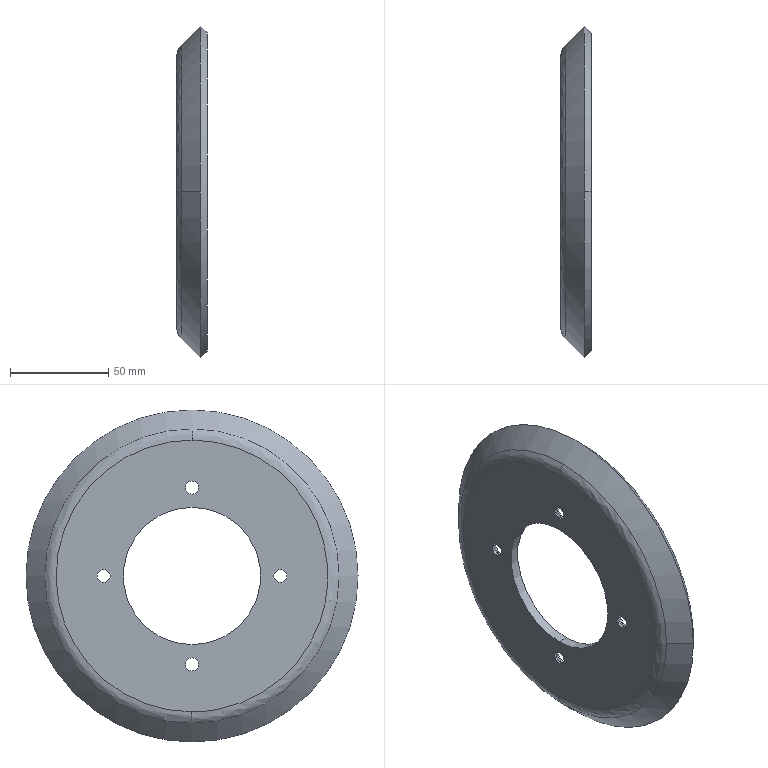Part | SolidWorks | features BaseBody 1 | 1 solid | 38 faces | box 15.556 x 169.042 x 169.042 mm | volume 97536 mm3 | cylinder 18 | cone 14 | spline 4 | plane 2 | commonest cylinder face diameters 6.6 x8 13 x8 70 x2